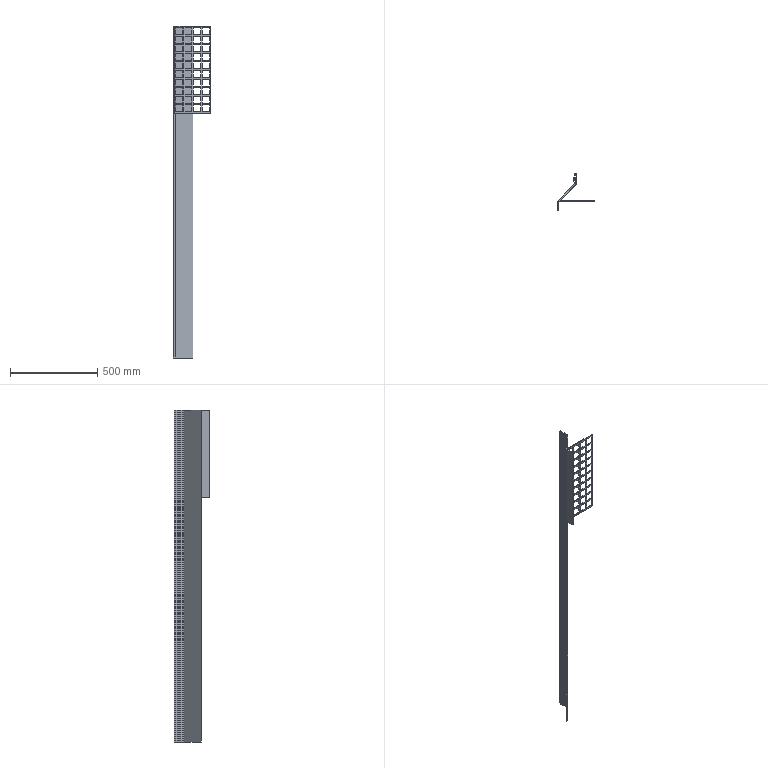Part | SolidWorks | features MirrorStock 1 | 2 solids | 195 faces | box 216 x 206 x 1900 mm | volume 3633510 mm3 | plane 195